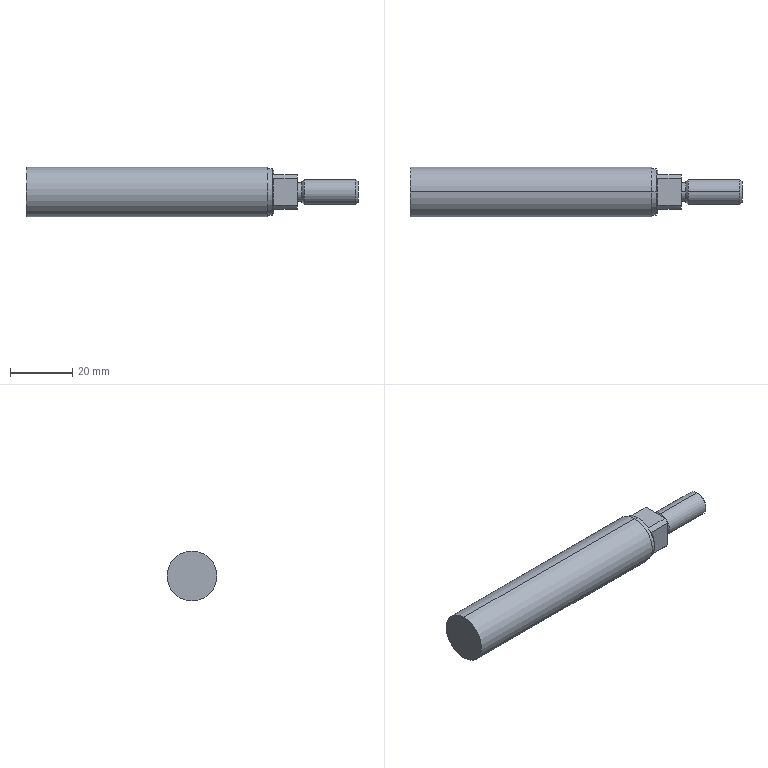Part | STEP file | Guide wheel mechanism revised.sldasm-Part-422 | 1 solid | 28 faces | box 106.5 x 16 x 16 mm | volume 17746 mm3 | plane 14 | cylinder 10 | cone 4 | commonest cylinder face diameters 6 x2 8 x2 14 x2 15 x2 16 x2
STEP:
#1=CARTESIAN_POINT('',(39.,0.,3.233));
#2=VERTEX_POINT('',#1);
#3=CARTESIAN_POINT('',(39.,0.,-3.233));
#4=VERTEX_POINT('',#3);
#5=CARTESIAN_POINT('',(39.,0.,0.));
#6=DIRECTION('',(-1.,0.,0.));
#7=DIRECTION('',(0.,0.,1.));
#8=AXIS2_PLACEMENT_3D('',#5,#6,#7);
#9=CIRCLE('',#8,3.233);
#10=EDGE_CURVE('',#2,#4,#9,.T.);
#11=ORIENTED_EDGE('',*,*,#10,.T.);
#12=CARTESIAN_POINT('',(38.233,0.,-4.));
#13=VERTEX_POINT('',#12);
#14=CARTESIAN_POINT('',(39.,0.,-3.233));
#15=DIRECTION('',(-0.7071,0.,-0.7071));
#16=VECTOR('',#15,1000.);
#17=LINE('',#14,#16);
#18=EDGE_CURVE('',#4,#13,#17,.T.);
#19=ORIENTED_EDGE('',*,*,#18,.T.);
#20=CARTESIAN_POINT('',(38.233,0.,4.));
#21=VERTEX_POINT('',#20);
#22=CARTESIAN_POINT('',(38.233,0.,0.));
#23=DIRECTION('',(-1.,0.,0.));
#24=DIRECTION('',(0.,0.,1.));
#25=AXIS2_PLACEMENT_3D('',#22,#23,#24);
#26=CIRCLE('',#25,4.);
#27=EDGE_CURVE('',#21,#13,#26,.T.);
#28=ORIENTED_EDGE('',*,*,#27,.F.);
#29=CARTESIAN_POINT('',(39.,0.,3.233));
#30=DIRECTION('',(-0.7071,0.,0.7071));
#31=VECTOR('',#30,1000.);
#32=LINE('',#29,#31);
#33=EDGE_CURVE('',#2,#21,#32,.T.);
#34=ORIENTED_EDGE('',*,*,#33,.F.);
#35=EDGE_LOOP('',(#11,#19,#28,#34));
#36=FACE_OUTER_BOUND('',#35,.T.);
#37=CARTESIAN_POINT('',(39.,0.,0.));
#38=DIRECTION('',(-1.,0.,0.));
#39=DIRECTION('',(0.,0.,1.));
#40=AXIS2_PLACEMENT_3D('',#37,#38,#39);
#41=CONICAL_SURFACE('',#40,3.233,0.7854);
#42=ADVANCED_FACE('',(#36),#41,.T.);
#43=ORIENTED_EDGE('',*,*,#27,.T.);
#44=CARTESIAN_POINT('',(21.767,0.,-4.));
#45=VERTEX_POINT('',#44);
#46=CARTESIAN_POINT('',(39.,0.,-4.));
#47=DIRECTION('',(-1.,0.,0.));
#48=VECTOR('',#47,1000.);
#49=LINE('',#46,#48);
#50=EDGE_CURVE('',#13,#45,#49,.T.);
#51=ORIENTED_EDGE('',*,*,#50,.T.);
#52=CARTESIAN_POINT('',(21.767,0.,4.));
#53=VERTEX_POINT('',#52);
#54=CARTESIAN_POINT('',(21.767,0.,0.));
#55=DIRECTION('',(-1.,0.,0.));
#56=DIRECTION('',(0.,0.,1.));
#57=AXIS2_PLACEMENT_3D('',#54,#55,#56);
#58=CIRCLE('',#57,4.);
#59=EDGE_CURVE('',#53,#45,#58,.T.);
#60=ORIENTED_EDGE('',*,*,#59,.F.);
#61=CARTESIAN_POINT('',(39.,0.,4.));
#62=DIRECTION('',(-1.,0.,0.));
#63=VECTOR('',#62,1000.);
#64=LINE('',#61,#63);
#65=EDGE_CURVE('',#21,#53,#64,.T.);
#66=ORIENTED_EDGE('',*,*,#65,.F.);
#67=EDGE_LOOP('',(#43,#51,#60,#66));
#68=FACE_OUTER_BOUND('',#67,.T.);
#69=CARTESIAN_POINT('',(39.,0.,0.));
#70=DIRECTION('',(-1.,0.,0.));
#71=DIRECTION('',(0.,0.,1.));
#72=AXIS2_PLACEMENT_3D('',#69,#70,#71);
#73=CYLINDRICAL_SURFACE('',#72,4.);
#74=ADVANCED_FACE('',(#68),#73,.T.);
#75=CARTESIAN_POINT('',(21.,0.,3.233));
#76=VERTEX_POINT('',#75);
#77=CARTESIAN_POINT('',(21.,0.,-3.233));
#78=VERTEX_POINT('',#77);
#79=CARTESIAN_POINT('',(21.,0.,0.));
#80=DIRECTION('',(-1.,0.,0.));
#81=DIRECTION('',(0.,0.,1.));
#82=AXIS2_PLACEMENT_3D('',#79,#80,#81);
#83=CIRCLE('',#82,3.233);
#84=EDGE_CURVE('',#76,#78,#83,.T.);
#85=ORIENTED_EDGE('',*,*,#84,.F.);
#86=CARTESIAN_POINT('',(21.767,0.,4.));
#87=DIRECTION('',(0.7071,0.,0.7071));
#88=VECTOR('',#87,1000.);
#89=LINE('',#86,#88);
#90=EDGE_CURVE('',#76,#53,#89,.T.);
#91=ORIENTED_EDGE('',*,*,#90,.T.);
#92=ORIENTED_EDGE('',*,*,#59,.T.);
#93=CARTESIAN_POINT('',(21.767,0.,-4.));
#94=DIRECTION('',(0.7071,0.,-0.7071));
#95=VECTOR('',#94,1000.);
#96=LINE('',#93,#95);
#97=EDGE_CURVE('',#78,#45,#96,.T.);
#98=ORIENTED_EDGE('',*,*,#97,.F.);
#99=EDGE_LOOP('',(#85,#91,#92,#98));
#100=FACE_OUTER_BOUND('',#99,.T.);
#101=CARTESIAN_POINT('',(21.767,0.,0.));
#102=DIRECTION('',(1.,0.,0.));
#103=DIRECTION('',(0.,0.,-1.));
#104=AXIS2_PLACEMENT_3D('',#101,#102,#103);
#105=CONICAL_SURFACE('',#104,4.,0.7854);
#106=ADVANCED_FACE('',(#100),#105,.T.);
#107=CARTESIAN_POINT('',(21.,0.,3.));
#108=VERTEX_POINT('',#107);
#109=CARTESIAN_POINT('',(21.,0.,-3.));
#110=VERTEX_POINT('',#109);
#111=CARTESIAN_POINT('',(21.,0.,0.));
#112=DIRECTION('',(-1.,0.,0.));
#113=DIRECTION('',(0.,0.,1.));
#114=AXIS2_PLACEMENT_3D('',#111,#112,#113);
#115=CIRCLE('',#114,3.);
#116=EDGE_CURVE('',#108,#110,#115,.T.);
#117=ORIENTED_EDGE('',*,*,#116,.T.);
#118=CARTESIAN_POINT('',(19.5,0.,-3.));
#119=VERTEX_POINT('',#118);
#120=CARTESIAN_POINT('',(39.,0.,-3.));
#121=DIRECTION('',(-1.,0.,0.));
#122=VECTOR('',#121,1000.);
#123=LINE('',#120,#122);
#124=EDGE_CURVE('',#110,#119,#123,.T.);
#125=ORIENTED_EDGE('',*,*,#124,.T.);
#126=CARTESIAN_POINT('',(19.5,0.,3.));
#127=VERTEX_POINT('',#126);
#128=CARTESIAN_POINT('',(19.5,0.,0.));
#129=DIRECTION('',(-1.,0.,0.));
#130=DIRECTION('',(0.,0.,1.));
#131=AXIS2_PLACEMENT_3D('',#128,#129,#130);
#132=CIRCLE('',#131,3.);
#133=EDGE_CURVE('',#127,#119,#132,.T.);
#134=ORIENTED_EDGE('',*,*,#133,.F.);
#135=CARTESIAN_POINT('',(39.,0.,3.));
#136=DIRECTION('',(-1.,0.,0.));
#137=VECTOR('',#136,1000.);
#138=LINE('',#135,#137);
#139=EDGE_CURVE('',#108,#127,#138,.T.);
#140=ORIENTED_EDGE('',*,*,#139,.F.);
#141=EDGE_LOOP('',(#117,#125,#134,#140));
#142=FACE_OUTER_BOUND('',#141,.T.);
#143=CARTESIAN_POINT('',(39.,0.,0.));
#144=DIRECTION('',(-1.,0.,0.));
#145=DIRECTION('',(0.,0.,1.));
#146=AXIS2_PLACEMENT_3D('',#143,#144,#145);
#147=CYLINDRICAL_SURFACE('',#146,3.);
#148=ADVANCED_FACE('',(#142),#147,.T.);
#149=CARTESIAN_POINT('',(11.5,0.,7.5));
#150=VERTEX_POINT('',#149);
#151=CARTESIAN_POINT('',(11.5,0.,-7.5));
#152=VERTEX_POINT('',#151);
#153=CARTESIAN_POINT('',(11.5,0.,0.));
#154=DIRECTION('',(-1.,0.,0.));
#155=DIRECTION('',(0.,0.,1.));
#156=AXIS2_PLACEMENT_3D('',#153,#154,#155);
#157=CIRCLE('',#156,7.5);
#158=EDGE_CURVE('',#150,#152,#157,.T.);
#159=ORIENTED_EDGE('',*,*,#158,.T.);
#160=CARTESIAN_POINT('',(10.,0.,-7.5));
#161=VERTEX_POINT('',#160);
#162=CARTESIAN_POINT('',(39.,0.,-7.5));
#163=DIRECTION('',(-1.,0.,0.));
#164=VECTOR('',#163,1000.);
#165=LINE('',#162,#164);
#166=EDGE_CURVE('',#152,#161,#165,.T.);
#167=ORIENTED_EDGE('',*,*,#166,.T.);
#168=CARTESIAN_POINT('',(10.,0.,7.5));
#169=VERTEX_POINT('',#168);
#170=CARTESIAN_POINT('',(10.,0.,0.));
#171=DIRECTION('',(-1.,0.,0.));
#172=DIRECTION('',(0.,0.,1.));
#173=AXIS2_PLACEMENT_3D('',#170,#171,#172);
#174=CIRCLE('',#173,7.5);
#175=EDGE_CURVE('',#169,#161,#174,.T.);
#176=ORIENTED_EDGE('',*,*,#175,.F.);
#177=CARTESIAN_POINT('',(39.,0.,7.5));
#178=DIRECTION('',(-1.,0.,0.));
#179=VECTOR('',#178,1000.);
#180=LINE('',#177,#179);
#181=EDGE_CURVE('',#150,#169,#180,.T.);
#182=ORIENTED_EDGE('',*,*,#181,.F.);
#183=EDGE_LOOP('',(#159,#167,#176,#182));
#184=FACE_OUTER_BOUND('',#183,.T.);
#185=CARTESIAN_POINT('',(39.,0.,0.));
#186=DIRECTION('',(-1.,0.,0.));
#187=DIRECTION('',(0.,0.,1.));
#188=AXIS2_PLACEMENT_3D('',#185,#186,#187);
#189=CYLINDRICAL_SURFACE('',#188,7.5);
#190=ADVANCED_FACE('',(#184),#189,.T.);
#191=CARTESIAN_POINT('',(10.,0.,8.));
#192=VERTEX_POINT('',#191);
#193=CARTESIAN_POINT('',(10.,0.,-8.));
#194=VERTEX_POINT('',#193);
#195=CARTESIAN_POINT('',(10.,0.,0.));
#196=DIRECTION('',(-1.,0.,0.));
#197=DIRECTION('',(0.,0.,1.));
#198=AXIS2_PLACEMENT_3D('',#195,#196,#197);
#199=CIRCLE('',#198,8.);
#200=EDGE_CURVE('',#192,#194,#199,.T.);
#201=ORIENTED_EDGE('',*,*,#200,.T.);
#202=CARTESIAN_POINT('',(-67.5,0.,-8.));
#203=VERTEX_POINT('',#202);
#204=CARTESIAN_POINT('',(39.,0.,-8.));
#205=DIRECTION('',(-1.,0.,0.));
#206=VECTOR('',#205,1000.);
#207=LINE('',#204,#206);
#208=EDGE_CURVE('',#194,#203,#207,.T.);
#209=ORIENTED_EDGE('',*,*,#208,.T.);
#210=CARTESIAN_POINT('',(-67.5,0.,8.));
#211=VERTEX_POINT('',#210);
#212=CARTESIAN_POINT('',(-67.5,0.,0.));
#213=DIRECTION('',(-1.,0.,0.));
#214=DIRECTION('',(0.,0.,1.));
#215=AXIS2_PLACEMENT_3D('',#212,#213,#214);
#216=CIRCLE('',#215,8.);
#217=EDGE_CURVE('',#211,#203,#216,.T.);
#218=ORIENTED_EDGE('',*,*,#217,.F.);
#219=CARTESIAN_POINT('',(39.,0.,8.));
#220=DIRECTION('',(-1.,0.,0.));
#221=VECTOR('',#220,1000.);
#222=LINE('',#219,#221);
#223=EDGE_CURVE('',#192,#211,#222,.T.);
#224=ORIENTED_EDGE('',*,*,#223,.F.);
#225=EDGE_LOOP('',(#201,#209,#218,#224));
#226=FACE_OUTER_BOUND('',#225,.T.);
#227=CARTESIAN_POINT('',(39.,0.,0.));
#228=DIRECTION('',(-1.,0.,0.));
#229=DIRECTION('',(0.,0.,1.));
#230=AXIS2_PLACEMENT_3D('',#227,#228,#229);
#231=CYLINDRICAL_SURFACE('',#230,8.);
#232=ADVANCED_FACE('',(#226),#231,.T.);
#233=CARTESIAN_POINT('',(12.,0.,-7.));
#234=VERTEX_POINT('',#233);
#235=CARTESIAN_POINT('',(12.,4.33,-5.5));
#236=VERTEX_POINT('',#235);
#237=CARTESIAN_POINT('',(12.,0.,0.));
#238=DIRECTION('',(1.,0.,0.));
#239=DIRECTION('',(0.,0.,-1.));
#240=AXIS2_PLACEMENT_3D('',#237,#238,#239);
#241=CIRCLE('',#240,7.);
#242=EDGE_CURVE('',#234,#236,#241,.T.);
#243=ORIENTED_EDGE('',*,*,#242,.F.);
#244=CARTESIAN_POINT('',(11.5,0.,-7.));
#245=VERTEX_POINT('',#244);
#246=CARTESIAN_POINT('',(39.,0.,-7.));
#247=DIRECTION('',(-1.,0.,0.));
#248=VECTOR('',#247,1000.);
#249=LINE('',#246,#248);
#250=EDGE_CURVE('',#234,#245,#249,.T.);
#251=ORIENTED_EDGE('',*,*,#250,.T.);
#252=CARTESIAN_POINT('',(11.5,0.,7.));
#253=VERTEX_POINT('',#252);
#254=CARTESIAN_POINT('',(11.5,0.,0.));
#255=DIRECTION('',(-1.,0.,0.));
#256=DIRECTION('',(0.,0.,1.));
#257=AXIS2_PLACEMENT_3D('',#254,#255,#256);
#258=CIRCLE('',#257,7.);
#259=EDGE_CURVE('',#253,#245,#258,.T.);
#260=ORIENTED_EDGE('',*,*,#259,.F.);
#261=CARTESIAN_POINT('',(12.,0.,7.));
#262=VERTEX_POINT('',#261);
#263=CARTESIAN_POINT('',(39.,0.,7.));
#264=DIRECTION('',(-1.,0.,0.));
#265=VECTOR('',#264,1000.);
#266=LINE('',#263,#265);
#267=EDGE_CURVE('',#262,#253,#266,.T.);
#268=ORIENTED_EDGE('',*,*,#267,.F.);
#269=CARTESIAN_POINT('',(12.,4.33,5.5));
#270=VERTEX_POINT('',#269);
#271=CARTESIAN_POINT('',(12.,0.,0.));
#272=DIRECTION('',(1.,0.,0.));
#273=DIRECTION('',(0.,0.,-1.));
#274=AXIS2_PLACEMENT_3D('',#271,#272,#273);
#275=CIRCLE('',#274,7.);
#276=EDGE_CURVE('',#270,#262,#275,.T.);
#277=ORIENTED_EDGE('',*,*,#276,.F.);
#278=CARTESIAN_POINT('',(19.5,4.33,5.5));
#279=VERTEX_POINT('',#278);
#280=CARTESIAN_POINT('',(39.,4.33,5.5));
#281=DIRECTION('',(-1.,0.,0.));
#282=VECTOR('',#281,1000.);
#283=LINE('',#280,#282);
#284=EDGE_CURVE('',#279,#270,#283,.T.);
#285=ORIENTED_EDGE('',*,*,#284,.F.);
#286=CARTESIAN_POINT('',(19.5,5.5,4.33));
#287=VERTEX_POINT('',#286);
#288=CARTESIAN_POINT('',(19.5,0.,0.));
#289=DIRECTION('',(-1.,0.,0.));
#290=DIRECTION('',(0.,0.,1.));
#291=AXIS2_PLACEMENT_3D('',#288,#289,#290);
#292=CIRCLE('',#291,7.);
#293=EDGE_CURVE('',#279,#287,#292,.T.);
#294=ORIENTED_EDGE('',*,*,#293,.T.);
#295=CARTESIAN_POINT('',(12.,5.5,4.33));
#296=VERTEX_POINT('',#295);
#297=CARTESIAN_POINT('',(39.,5.5,4.33));
#298=DIRECTION('',(1.,0.,0.));
#299=VECTOR('',#298,1000.);
#300=LINE('',#297,#299);
#301=EDGE_CURVE('',#296,#287,#300,.T.);
#302=ORIENTED_EDGE('',*,*,#301,.F.);
#303=CARTESIAN_POINT('',(12.,5.5,-4.33));
#304=VERTEX_POINT('',#303);
#305=CARTESIAN_POINT('',(12.,0.,0.));
#306=DIRECTION('',(1.,0.,0.));
#307=DIRECTION('',(0.,0.,-1.));
#308=AXIS2_PLACEMENT_3D('',#305,#306,#307);
#309=CIRCLE('',#308,7.);
#310=EDGE_CURVE('',#304,#296,#309,.T.);
#311=ORIENTED_EDGE('',*,*,#310,.F.);
#312=CARTESIAN_POINT('',(19.5,5.5,-4.33));
#313=VERTEX_POINT('',#312);
#314=CARTESIAN_POINT('',(39.,5.5,-4.33));
#315=DIRECTION('',(-1.,0.,0.));
#316=VECTOR('',#315,1000.);
#317=LINE('',#314,#316);
#318=EDGE_CURVE('',#313,#304,#317,.T.);
#319=ORIENTED_EDGE('',*,*,#318,.F.);
#320=CARTESIAN_POINT('',(19.5,4.33,-5.5));
#321=VERTEX_POINT('',#320);
#322=CARTESIAN_POINT('',(19.5,0.,0.));
#323=DIRECTION('',(-1.,0.,0.));
#324=DIRECTION('',(0.,0.,1.));
#325=AXIS2_PLACEMENT_3D('',#322,#323,#324);
#326=CIRCLE('',#325,7.);
#327=EDGE_CURVE('',#313,#321,#326,.T.);
#328=ORIENTED_EDGE('',*,*,#327,.T.);
#329=CARTESIAN_POINT('',(39.,4.33,-5.5));
#330=DIRECTION('',(1.,0.,0.));
#331=VECTOR('',#330,1000.);
#332=LINE('',#329,#331);
#333=EDGE_CURVE('',#236,#321,#332,.T.);
#334=ORIENTED_EDGE('',*,*,#333,.F.);
#335=EDGE_LOOP('',(#243,#251,#260,#268,#277,#285,#294,#302,#311,#319,#328,#334));
#336=FACE_OUTER_BOUND('',#335,.T.);
#337=CARTESIAN_POINT('',(39.,0.,0.));
#338=DIRECTION('',(-1.,0.,0.));
#339=DIRECTION('',(0.,0.,1.));
#340=AXIS2_PLACEMENT_3D('',#337,#338,#339);
#341=CYLINDRICAL_SURFACE('',#340,7.);
#342=ADVANCED_FACE('',(#336),#341,.T.);
#343=ORIENTED_EDGE('',*,*,#250,.F.);
#344=CARTESIAN_POINT('',(12.,-4.33,-5.5));
#345=VERTEX_POINT('',#344);
#346=CARTESIAN_POINT('',(12.,0.,0.));
#347=DIRECTION('',(1.,0.,0.));
#348=DIRECTION('',(0.,0.,-1.));
#349=AXIS2_PLACEMENT_3D('',#346,#347,#348);
#350=CIRCLE('',#349,7.);
#351=EDGE_CURVE('',#345,#234,#350,.T.);
#352=ORIENTED_EDGE('',*,*,#351,.F.);
#353=CARTESIAN_POINT('',(19.5,-4.33,-5.5));
#354=VERTEX_POINT('',#353);
#355=CARTESIAN_POINT('',(39.,-4.33,-5.5));
#356=DIRECTION('',(-1.,0.,0.));
#357=VECTOR('',#356,1000.);
#358=LINE('',#355,#357);
#359=EDGE_CURVE('',#354,#345,#358,.T.);
#360=ORIENTED_EDGE('',*,*,#359,.F.);
#361=CARTESIAN_POINT('',(19.5,-5.5,-4.33));
#362=VERTEX_POINT('',#361);
#363=CARTESIAN_POINT('',(19.5,0.,0.));
#364=DIRECTION('',(-1.,0.,0.));
#365=DIRECTION('',(0.,0.,1.));
#366=AXIS2_PLACEMENT_3D('',#363,#364,#365);
#367=CIRCLE('',#366,7.);
#368=EDGE_CURVE('',#354,#362,#367,.T.);
#369=ORIENTED_EDGE('',*,*,#368,.T.);
#370=CARTESIAN_POINT('',(12.,-5.5,-4.33));
#371=VERTEX_POINT('',#370);
#372=CARTESIAN_POINT('',(39.,-5.5,-4.33));
#373=DIRECTION('',(1.,0.,0.));
#374=VECTOR('',#373,1000.);
#375=LINE('',#372,#374);
#376=EDGE_CURVE('',#371,#362,#375,.T.);
#377=ORIENTED_EDGE('',*,*,#376,.F.);
#378=CARTESIAN_POINT('',(12.,-5.5,4.33));
#379=VERTEX_POINT('',#378);
#380=CARTESIAN_POINT('',(12.,0.,0.));
#381=DIRECTION('',(1.,0.,0.));
#382=DIRECTION('',(0.,0.,-1.));
#383=AXIS2_PLACEMENT_3D('',#380,#381,#382);
#384=CIRCLE('',#383,7.);
#385=EDGE_CURVE('',#379,#371,#384,.T.);
#386=ORIENTED_EDGE('',*,*,#385,.F.);
#387=CARTESIAN_POINT('',(19.5,-5.5,4.33));
#388=VERTEX_POINT('',#387);
#389=CARTESIAN_POINT('',(39.,-5.5,4.33));
#390=DIRECTION('',(-1.,0.,0.));
#391=VECTOR('',#390,1000.);
#392=LINE('',#389,#391);
#393=EDGE_CURVE('',#388,#379,#392,.T.);
#394=ORIENTED_EDGE('',*,*,#393,.F.);
#395=CARTESIAN_POINT('',(19.5,-4.33,5.5));
#396=VERTEX_POINT('',#395);
#397=CARTESIAN_POINT('',(19.5,0.,0.));
#398=DIRECTION('',(-1.,0.,0.));
#399=DIRECTION('',(0.,0.,1.));
#400=AXIS2_PLACEMENT_3D('',#397,#398,#399);
#401=CIRCLE('',#400,7.);
#402=EDGE_CURVE('',#388,#396,#401,.T.);
#403=ORIENTED_EDGE('',*,*,#402,.T.);
#404=CARTESIAN_POINT('',(12.,-4.33,5.5));
#405=VERTEX_POINT('',#404);
#406=CARTESIAN_POINT('',(39.,-4.33,5.5));
#407=DIRECTION('',(1.,0.,0.));
#408=VECTOR('',#407,1000.);
#409=LINE('',#406,#408);
#410=EDGE_CURVE('',#405,#396,#409,.T.);
#411=ORIENTED_EDGE('',*,*,#410,.F.);
#412=CARTESIAN_POINT('',(12.,0.,0.));
#413=DIRECTION('',(1.,0.,0.));
#414=DIRECTION('',(0.,0.,-1.));
#415=AXIS2_PLACEMENT_3D('',#412,#413,#414);
#416=CIRCLE('',#415,7.);
#417=EDGE_CURVE('',#262,#405,#416,.T.);
#418=ORIENTED_EDGE('',*,*,#417,.F.);
#419=ORIENTED_EDGE('',*,*,#267,.T.);
#420=CARTESIAN_POINT('',(11.5,0.,0.));
#421=DIRECTION('',(-1.,0.,0.));
#422=DIRECTION('',(0.,0.,1.));
#423=AXIS2_PLACEMENT_3D('',#420,#421,#422);
#424=CIRCLE('',#423,7.);
#425=EDGE_CURVE('',#245,#253,#424,.T.);
#426=ORIENTED_EDGE('',*,*,#425,.F.);
#427=EDGE_LOOP('',(#343,#352,#360,#369,#377,#386,#394,#403,#411,#418,#419,#426));
#428=FACE_OUTER_BOUND('',#427,.T.);
#429=CARTESIAN_POINT('',(39.,0.,0.));
#430=DIRECTION('',(-1.,0.,0.));
#431=DIRECTION('',(0.,0.,1.));
#432=AXIS2_PLACEMENT_3D('',#429,#430,#431);
#433=CYLINDRICAL_SURFACE('',#432,7.);
#434=ADVANCED_FACE('',(#428),#433,.T.);
#435=ORIENTED_EDGE('',*,*,#133,.T.);
#436=CARTESIAN_POINT('',(19.5,0.,0.));
#437=DIRECTION('',(-1.,0.,0.));
#438=DIRECTION('',(0.,0.,1.));
#439=AXIS2_PLACEMENT_3D('',#436,#437,#438);
#440=CIRCLE('',#439,3.);
#441=EDGE_CURVE('',#119,#127,#440,.T.);
#442=ORIENTED_EDGE('',*,*,#441,.T.);
#443=EDGE_LOOP('',(#435,#442));
#444=FACE_BOUND('',#443,.T.);
#445=CARTESIAN_POINT('',(19.5,5.5,0.));
#446=DIRECTION('',(0.,0.,-1.));
#447=VECTOR('',#446,1000.);
#448=LINE('',#445,#447);
#449=EDGE_CURVE('',#287,#313,#448,.T.);
#450=ORIENTED_EDGE('',*,*,#449,.F.);
#451=ORIENTED_EDGE('',*,*,#293,.F.);
#452=CARTESIAN_POINT('',(19.5,7.,5.5));
#453=DIRECTION('',(0.,1.,0.));
#454=VECTOR('',#453,1000.);
#455=LINE('',#452,#454);
#456=EDGE_CURVE('',#396,#279,#455,.T.);
#457=ORIENTED_EDGE('',*,*,#456,.F.);
#458=ORIENTED_EDGE('',*,*,#402,.F.);
#459=CARTESIAN_POINT('',(19.5,-5.5,0.));
#460=DIRECTION('',(0.,0.,1.));
#461=VECTOR('',#460,1000.);
#462=LINE('',#459,#461);
#463=EDGE_CURVE('',#362,#388,#462,.T.);
#464=ORIENTED_EDGE('',*,*,#463,.F.);
#465=ORIENTED_EDGE('',*,*,#368,.F.);
#466=CARTESIAN_POINT('',(19.5,7.,-5.5));
#467=DIRECTION('',(0.,-1.,0.));
#468=VECTOR('',#467,1000.);
#469=LINE('',#466,#468);
#470=EDGE_CURVE('',#321,#354,#469,.T.);
#471=ORIENTED_EDGE('',*,*,#470,.F.);
#472=ORIENTED_EDGE('',*,*,#327,.F.);
#473=EDGE_LOOP('',(#450,#451,#457,#458,#464,#465,#471,#472));
#474=FACE_OUTER_BOUND('',#473,.T.);
#475=CARTESIAN_POINT('',(19.5,7.,0.));
#476=DIRECTION('',(-1.,0.,0.));
#477=DIRECTION('',(0.,0.,1.));
#478=AXIS2_PLACEMENT_3D('',#475,#476,#477);
#479=PLANE('',#478);
#480=ADVANCED_FACE('',(#444,#474),#479,.F.);
#481=ORIENTED_EDGE('',*,*,#217,.T.);
#482=CARTESIAN_POINT('',(-67.5,0.,0.));
#483=DIRECTION('',(-1.,0.,0.));
#484=DIRECTION('',(0.,0.,1.));
#485=AXIS2_PLACEMENT_3D('',#482,#483,#484);
#486=CIRCLE('',#485,8.);
#487=EDGE_CURVE('',#203,#211,#486,.T.);
#488=ORIENTED_EDGE('',*,*,#487,.T.);
#489=EDGE_LOOP('',(#481,#488));
#490=FACE_OUTER_BOUND('',#489,.T.);
#491=CARTESIAN_POINT('',(-67.5,0.,0.));
#492=DIRECTION('',(1.,0.,0.));
#493=DIRECTION('',(0.,0.,-1.));
#494=AXIS2_PLACEMENT_3D('',#491,#492,#493);
#495=PLANE('',#494);
#496=ADVANCED_FACE('',(#490),#495,.F.);
#497=ORIENTED_EDGE('',*,*,#208,.F.);
#498=CARTESIAN_POINT('',(10.,0.,0.));
#499=DIRECTION('',(-1.,0.,0.));
#500=DIRECTION('',(0.,0.,1.));
#501=AXIS2_PLACEMENT_3D('',#498,#499,#500);
#502=CIRCLE('',#501,8.);
#503=EDGE_CURVE('',#194,#192,#502,.T.);
#504=ORIENTED_EDGE('',*,*,#503,.T.);
#505=ORIENTED_EDGE('',*,*,#223,.T.);
#506=ORIENTED_EDGE('',*,*,#487,.F.);
#507=EDGE_LOOP('',(#497,#504,#505,#506));
#508=FACE_OUTER_BOUND('',#507,.T.);
#509=CARTESIAN_POINT('',(39.,0.,0.));
#510=DIRECTION('',(-1.,0.,0.));
#511=DIRECTION('',(0.,0.,1.));
#512=AXIS2_PLACEMENT_3D('',#509,#510,#511);
#513=CYLINDRICAL_SURFACE('',#512,8.);
#514=ADVANCED_FACE('',(#508),#513,.T.);
#515=ORIENTED_EDGE('',*,*,#200,.F.);
#516=ORIENTED_EDGE('',*,*,#503,.F.);
#517=EDGE_LOOP('',(#515,#516));
#518=FACE_OUTER_BOUND('',#517,.T.);
#519=ORIENTED_EDGE('',*,*,#175,.T.);
#520=CARTESIAN_POINT('',(10.,0.,0.));
#521=DIRECTION('',(-1.,0.,0.));
#522=DIRECTION('',(0.,0.,1.));
#523=AXIS2_PLACEMENT_3D('',#520,#521,#522);
#524=CIRCLE('',#523,7.5);
#525=EDGE_CURVE('',#161,#169,#524,.T.);
#526=ORIENTED_EDGE('',*,*,#525,.T.);
#527=EDGE_LOOP('',(#519,#526));
#528=FACE_BOUND('',#527,.T.);
#529=CARTESIAN_POINT('',(10.,8.,0.));
#530=DIRECTION('',(-1.,0.,0.));
#531=DIRECTION('',(0.,0.,1.));
#532=AXIS2_PLACEMENT_3D('',#529,#530,#531);
#533=PLANE('',#532);
#534=ADVANCED_FACE('',(#518,#528),#533,.F.);
#535=ORIENTED_EDGE('',*,*,#166,.F.);
#536=CARTESIAN_POINT('',(11.5,0.,0.));
#537=DIRECTION('',(-1.,0.,0.));
#538=DIRECTION('',(0.,0.,1.));
#539=AXIS2_PLACEMENT_3D('',#536,#537,#538);
#540=CIRCLE('',#539,7.5);
#541=EDGE_CURVE('',#152,#150,#540,.T.);
#542=ORIENTED_EDGE('',*,*,#541,.T.);
#543=ORIENTED_EDGE('',*,*,#181,.T.);
#544=ORIENTED_EDGE('',*,*,#525,.F.);
#545=EDGE_LOOP('',(#535,#542,#543,#544));
#546=FACE_OUTER_BOUND('',#545,.T.);
#547=CARTESIAN_POINT('',(39.,0.,0.));
#548=DIRECTION('',(-1.,0.,0.));
#549=DIRECTION('',(0.,0.,1.));
#550=AXIS2_PLACEMENT_3D('',#547,#548,#549);
#551=CYLINDRICAL_SURFACE('',#550,7.5);
#552=ADVANCED_FACE('',(#546),#551,.T.);
#553=ORIENTED_EDGE('',*,*,#158,.F.);
#554=ORIENTED_EDGE('',*,*,#541,.F.);
#555=EDGE_LOOP('',(#553,#554));
#556=FACE_OUTER_BOUND('',#555,.T.);
#557=ORIENTED_EDGE('',*,*,#259,.T.);
#558=ORIENTED_EDGE('',*,*,#425,.T.);
#559=EDGE_LOOP('',(#557,#558));
#560=FACE_BOUND('',#559,.T.);
#561=CARTESIAN_POINT('',(11.5,7.5,0.));
#562=DIRECTION('',(-1.,0.,0.));
#563=DIRECTION('',(0.,0.,1.));
#564=AXIS2_PLACEMENT_3D('',#561,#562,#563);
#565=PLANE('',#564);
#566=ADVANCED_FACE('',(#556,#560),#565,.F.);
#567=ORIENTED_EDGE('',*,*,#124,.F.);
#568=CARTESIAN_POINT('',(21.,0.,0.));
#569=DIRECTION('',(-1.,0.,0.));
#570=DIRECTION('',(0.,0.,1.));
#571=AXIS2_PLACEMENT_3D('',#568,#569,#570);
#572=CIRCLE('',#571,3.);
#573=EDGE_CURVE('',#110,#108,#572,.T.);
#574=ORIENTED_EDGE('',*,*,#573,.T.);
#575=ORIENTED_EDGE('',*,*,#139,.T.);
#576=ORIENTED_EDGE('',*,*,#441,.F.);
#577=EDGE_LOOP('',(#567,#574,#575,#576));
#578=FACE_OUTER_BOUND('',#577,.T.);
#579=CARTESIAN_POINT('',(39.,0.,0.));
#580=DIRECTION('',(-1.,0.,0.));
#581=DIRECTION('',(0.,0.,1.));
#582=AXIS2_PLACEMENT_3D('',#579,#580,#581);
#583=CYLINDRICAL_SURFACE('',#582,3.);
#584=ADVANCED_FACE('',(#578),#583,.T.);
#585=ORIENTED_EDGE('',*,*,#116,.F.);
#586=ORIENTED_EDGE('',*,*,#573,.F.);
#587=EDGE_LOOP('',(#585,#586));
#588=FACE_BOUND('',#587,.T.);
#589=CARTESIAN_POINT('',(21.,0.,0.));
#590=DIRECTION('',(-1.,0.,0.));
#591=DIRECTION('',(0.,0.,1.));
#592=AXIS2_PLACEMENT_3D('',#589,#590,#591);
#593=CIRCLE('',#592,3.233);
#594=EDGE_CURVE('',#78,#76,#593,.T.);
#595=ORIENTED_EDGE('',*,*,#594,.T.);
#596=ORIENTED_EDGE('',*,*,#84,.T.);
#597=EDGE_LOOP('',(#595,#596));
#598=FACE_OUTER_BOUND('',#597,.T.);
#599=CARTESIAN_POINT('',(21.,3.,0.));
#600=DIRECTION('',(1.,0.,0.));
#601=DIRECTION('',(0.,0.,-1.));
#602=AXIS2_PLACEMENT_3D('',#599,#600,#601);
#603=PLANE('',#602);
#604=ADVANCED_FACE('',(#588,#598),#603,.F.);
#605=ORIENTED_EDGE('',*,*,#90,.F.);
#606=ORIENTED_EDGE('',*,*,#594,.F.);
#607=ORIENTED_EDGE('',*,*,#97,.T.);
#608=CARTESIAN_POINT('',(21.767,0.,0.));
#609=DIRECTION('',(-1.,0.,0.));
#610=DIRECTION('',(0.,0.,1.));
#611=AXIS2_PLACEMENT_3D('',#608,#609,#610);
#612=CIRCLE('',#611,4.);
#613=EDGE_CURVE('',#45,#53,#612,.T.);
#614=ORIENTED_EDGE('',*,*,#613,.T.);
#615=EDGE_LOOP('',(#605,#606,#607,#614));
#616=FACE_OUTER_BOUND('',#615,.T.);
#617=CARTESIAN_POINT('',(21.767,0.,0.));
#618=DIRECTION('',(1.,0.,0.));
#619=DIRECTION('',(0.,0.,-1.));
#620=AXIS2_PLACEMENT_3D('',#617,#618,#619);
#621=CONICAL_SURFACE('',#620,4.,0.7854);
#622=ADVANCED_FACE('',(#616),#621,.T.);
#623=ORIENTED_EDGE('',*,*,#50,.F.);
#624=CARTESIAN_POINT('',(38.233,0.,0.));
#625=DIRECTION('',(-1.,0.,0.));
#626=DIRECTION('',(0.,0.,1.));
#627=AXIS2_PLACEMENT_3D('',#624,#625,#626);
#628=CIRCLE('',#627,4.);
#629=EDGE_CURVE('',#13,#21,#628,.T.);
#630=ORIENTED_EDGE('',*,*,#629,.T.);
#631=ORIENTED_EDGE('',*,*,#65,.T.);
#632=ORIENTED_EDGE('',*,*,#613,.F.);
#633=EDGE_LOOP('',(#623,#630,#631,#632));
#634=FACE_OUTER_BOUND('',#633,.T.);
#635=CARTESIAN_POINT('',(39.,0.,0.));
#636=DIRECTION('',(-1.,0.,0.));
#637=DIRECTION('',(0.,0.,1.));
#638=AXIS2_PLACEMENT_3D('',#635,#636,#637);
#639=CYLINDRICAL_SURFACE('',#638,4.);
#640=ADVANCED_FACE('',(#634),#639,.T.);
#641=ORIENTED_EDGE('',*,*,#18,.F.);
#642=CARTESIAN_POINT('',(39.,0.,0.));
#643=DIRECTION('',(-1.,0.,0.));
#644=DIRECTION('',(0.,0.,1.));
#645=AXIS2_PLACEMENT_3D('',#642,#643,#644);
#646=CIRCLE('',#645,3.233);
#647=EDGE_CURVE('',#4,#2,#646,.T.);
#648=ORIENTED_EDGE('',*,*,#647,.T.);
#649=ORIENTED_EDGE('',*,*,#33,.T.);
#650=ORIENTED_EDGE('',*,*,#629,.F.);
#651=EDGE_LOOP('',(#641,#648,#649,#650));
#652=FACE_OUTER_BOUND('',#651,.T.);
#653=CARTESIAN_POINT('',(39.,0.,0.));
#654=DIRECTION('',(-1.,0.,0.));
#655=DIRECTION('',(0.,0.,1.));
#656=AXIS2_PLACEMENT_3D('',#653,#654,#655);
#657=CONICAL_SURFACE('',#656,3.233,0.7854);
#658=ADVANCED_FACE('',(#652),#657,.T.);
#659=ORIENTED_EDGE('',*,*,#10,.F.);
#660=ORIENTED_EDGE('',*,*,#647,.F.);
#661=EDGE_LOOP('',(#659,#660));
#662=FACE_OUTER_BOUND('',#661,.T.);
#663=CARTESIAN_POINT('',(39.,3.233,0.));
#664=DIRECTION('',(-1.,0.,0.));
#665=DIRECTION('',(0.,0.,1.));
#666=AXIS2_PLACEMENT_3D('',#663,#664,#665);
#667=PLANE('',#666);
#668=ADVANCED_FACE('',(#662),#667,.F.);
#669=ORIENTED_EDGE('',*,*,#284,.T.);
#670=CARTESIAN_POINT('',(12.,5.5,5.5));
#671=DIRECTION('',(0.,-1.,0.));
#672=VECTOR('',#671,1000.);
#673=LINE('',#670,#672);
#674=EDGE_CURVE('',#270,#405,#673,.T.);
#675=ORIENTED_EDGE('',*,*,#674,.T.);
#676=ORIENTED_EDGE('',*,*,#410,.T.);
#677=ORIENTED_EDGE('',*,*,#456,.T.);
#678=EDGE_LOOP('',(#669,#675,#676,#677));
#679=FACE_OUTER_BOUND('',#678,.T.);
#680=CARTESIAN_POINT('',(12.,5.5,5.5));
#681=DIRECTION('',(0.,0.,1.));
#682=DIRECTION('',(1.,0.,0.));
#683=AXIS2_PLACEMENT_3D('',#680,#681,#682);
#684=PLANE('',#683);
#685=ADVANCED_FACE('',(#679),#684,.T.);
#686=ORIENTED_EDGE('',*,*,#276,.T.);
#687=ORIENTED_EDGE('',*,*,#417,.T.);
#688=ORIENTED_EDGE('',*,*,#674,.F.);
#689=EDGE_LOOP('',(#686,#687,#688));
#690=FACE_OUTER_BOUND('',#689,.T.);
#691=CARTESIAN_POINT('',(12.,0.,0.));
#692=DIRECTION('',(1.,0.,0.));
#693=DIRECTION('',(0.,0.,-1.));
#694=AXIS2_PLACEMENT_3D('',#691,#692,#693);
#695=PLANE('',#694);
#696=ADVANCED_FACE('',(#690),#695,.T.);
#697=ORIENTED_EDGE('',*,*,#393,.T.);
#698=CARTESIAN_POINT('',(12.,-5.5,5.5));
#699=DIRECTION('',(0.,0.,-1.));
#700=VECTOR('',#699,1000.);
#701=LINE('',#698,#700);
#702=EDGE_CURVE('',#379,#371,#701,.T.);
#703=ORIENTED_EDGE('',*,*,#702,.T.);
#704=ORIENTED_EDGE('',*,*,#376,.T.);
#705=ORIENTED_EDGE('',*,*,#463,.T.);
#706=EDGE_LOOP('',(#697,#703,#704,#705));
#707=FACE_OUTER_BOUND('',#706,.T.);
#708=CARTESIAN_POINT('',(12.,-5.5,5.5));
#709=DIRECTION('',(0.,-1.,0.));
#710=DIRECTION('',(0.,0.,-1.));
#711=AXIS2_PLACEMENT_3D('',#708,#709,#710);
#712=PLANE('',#711);
#713=ADVANCED_FACE('',(#707),#712,.T.);
#714=ORIENTED_EDGE('',*,*,#385,.T.);
#715=ORIENTED_EDGE('',*,*,#702,.F.);
#716=EDGE_LOOP('',(#714,#715));
#717=FACE_OUTER_BOUND('',#716,.T.);
#718=CARTESIAN_POINT('',(12.,0.,0.));
#719=DIRECTION('',(1.,0.,0.));
#720=DIRECTION('',(0.,0.,-1.));
#721=AXIS2_PLACEMENT_3D('',#718,#719,#720);
#722=PLANE('',#721);
#723=ADVANCED_FACE('',(#717),#722,.T.);
#724=ORIENTED_EDGE('',*,*,#359,.T.);
#725=CARTESIAN_POINT('',(12.,-5.5,-5.5));
#726=DIRECTION('',(0.,1.,0.));
#727=VECTOR('',#726,1000.);
#728=LINE('',#725,#727);
#729=EDGE_CURVE('',#345,#236,#728,.T.);
#730=ORIENTED_EDGE('',*,*,#729,.T.);
#731=ORIENTED_EDGE('',*,*,#333,.T.);
#732=ORIENTED_EDGE('',*,*,#470,.T.);
#733=EDGE_LOOP('',(#724,#730,#731,#732));
#734=FACE_OUTER_BOUND('',#733,.T.);
#735=CARTESIAN_POINT('',(12.,-5.5,-5.5));
#736=DIRECTION('',(0.,0.,-1.));
#737=DIRECTION('',(-1.,0.,0.));
#738=AXIS2_PLACEMENT_3D('',#735,#736,#737);
#739=PLANE('',#738);
#740=ADVANCED_FACE('',(#734),#739,.T.);
#741=ORIENTED_EDGE('',*,*,#351,.T.);
#742=ORIENTED_EDGE('',*,*,#242,.T.);
#743=ORIENTED_EDGE('',*,*,#729,.F.);
#744=EDGE_LOOP('',(#741,#742,#743));
#745=FACE_OUTER_BOUND('',#744,.T.);
#746=CARTESIAN_POINT('',(12.,0.,0.));
#747=DIRECTION('',(1.,0.,0.));
#748=DIRECTION('',(0.,0.,-1.));
#749=AXIS2_PLACEMENT_3D('',#746,#747,#748);
#750=PLANE('',#749);
#751=ADVANCED_FACE('',(#745),#750,.T.);
#752=ORIENTED_EDGE('',*,*,#310,.T.);
#753=CARTESIAN_POINT('',(12.,5.5,-5.5));
#754=DIRECTION('',(0.,0.,1.));
#755=VECTOR('',#754,1000.);
#756=LINE('',#753,#755);
#757=EDGE_CURVE('',#304,#296,#756,.T.);
#758=ORIENTED_EDGE('',*,*,#757,.F.);
#759=EDGE_LOOP('',(#752,#758));
#760=FACE_OUTER_BOUND('',#759,.T.);
#761=CARTESIAN_POINT('',(12.,0.,0.));
#762=DIRECTION('',(1.,0.,0.));
#763=DIRECTION('',(0.,0.,-1.));
#764=AXIS2_PLACEMENT_3D('',#761,#762,#763);
#765=PLANE('',#764);
#766=ADVANCED_FACE('',(#760),#765,.T.);
#767=ORIENTED_EDGE('',*,*,#318,.T.);
#768=ORIENTED_EDGE('',*,*,#757,.T.);
#769=ORIENTED_EDGE('',*,*,#301,.T.);
#770=ORIENTED_EDGE('',*,*,#449,.T.);
#771=EDGE_LOOP('',(#767,#768,#769,#770));
#772=FACE_OUTER_BOUND('',#771,.T.);
#773=CARTESIAN_POINT('',(12.,5.5,-5.5));
#774=DIRECTION('',(0.,1.,0.));
#775=DIRECTION('',(0.,0.,1.));
#776=AXIS2_PLACEMENT_3D('',#773,#774,#775);
#777=PLANE('',#776);
#778=ADVANCED_FACE('',(#772),#777,.T.);
#779=CLOSED_SHELL('',(#42,#74,#106,#148,#190,#232,#342,#434,#480,#496,#514,#534,#552,#566,#584,#604,#622,#640,#658,#668,#685,#696,#713,#723,#740,#751,#766,#778));
#780=MANIFOLD_SOLID_BREP('',#779);
#781=CARTESIAN_POINT('',(0.,0.,0.));
#782=DIRECTION('',(0.,0.,1.));
#783=DIRECTION('',(1.,0.,0.));
#784=AXIS2_PLACEMENT_3D('',#781,#782,#783);
#785=(LENGTH_UNIT()NAMED_UNIT(*)SI_UNIT(.MILLI.,.METRE.));
#786=UNCERTAINTY_MEASURE_WITH_UNIT(LENGTH_MEASURE(0.00001),#785,'','');
#787=(NAMED_UNIT(*)PLANE_ANGLE_UNIT()SI_UNIT($,.RADIAN.));
#788=(NAMED_UNIT(*)SI_UNIT($,.STERADIAN.)SOLID_ANGLE_UNIT());
#789=(GEOMETRIC_REPRESENTATION_CONTEXT(3)GLOBAL_UNCERTAINTY_ASSIGNED_CONTEXT((#786))GLOBAL_UNIT_ASSIGNED_CONTEXT((#785,#787,#788))REPRESENTATION_CONTEXT('',''));
#790=ADVANCED_BREP_SHAPE_REPRESENTATION('',(#780,#784),#789);